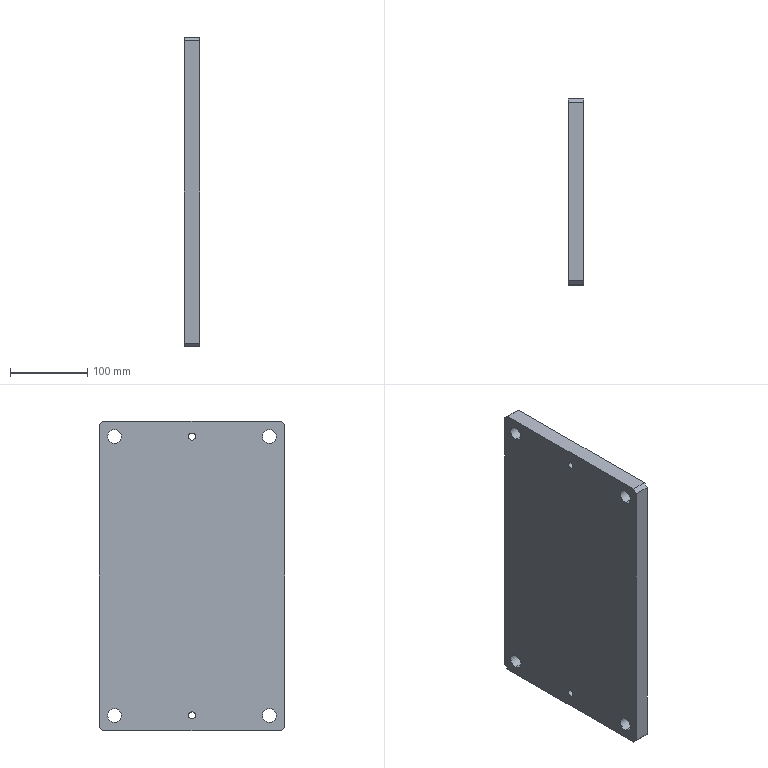Part | STEP file | Positioning_id934_x_t | 1 solid | 22 faces | box 20 x 240 x 400 mm | volume 1896098 mm3 | cylinder 12 | plane 10 | commonest cylinder face diameters 18 x8 9 x4